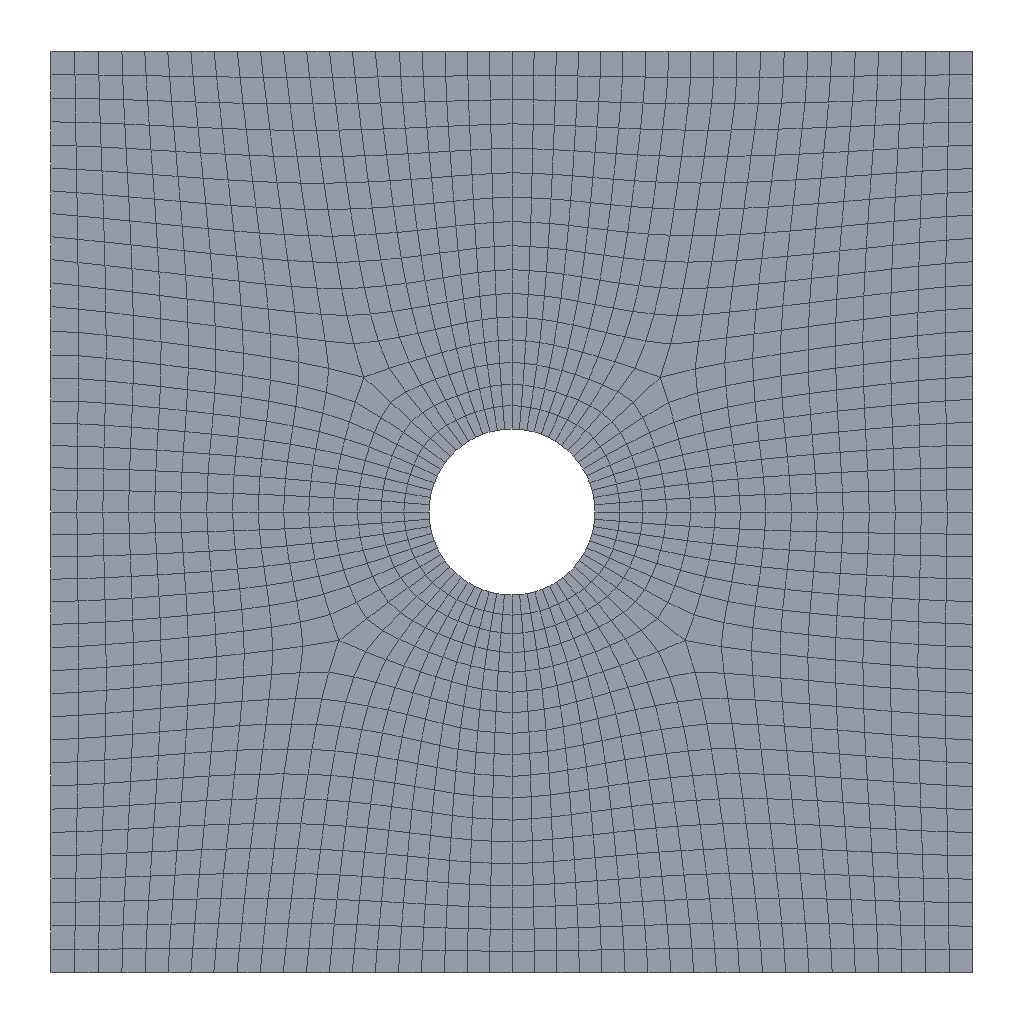Simulation study | abaqus
Set-up summary:
category,name,step,type,value,unit,region
solver,abaqus
solver,version,,,Abaqus/Standard 2020
units,not stated in the deck,,not stated
analysis,deck,,soils,soils
load_step,Step-1,Step-1,soils
load_step,requested,,,1
mesh,nodes,,,1736
mesh,elements,,,1622
element_type,CPE4P,,plane,1622
load,load commands in deck,,count,1
bc,support commands in deck,,count,2
material,MATERIAL-1,,in results
check,setup vs results,,match,"per instance, exact: element labels, types and connectivity; labels of the nodes the elements use; coordinates of those nodes at SINGLE_PRECISION in 1 of 1 instance(s)"
Abaqus input file, long lists of numbers shortened:
*Heading
** Job name: Job-1 Model name: Model-1
** Generated by: Abaqus/CAE 2020
*Preprint, echo=NO, model=NO, history=NO, contact=NO
**
** PARTS
**
*Part, name=Part-1
*Node
      1,        -400.,       -1200.
      2,        -400.,        -708.
** (1734 more lines like these left out)
*Element, type=CPE4P
  1,  88,  89, 330, 310
  2,  89,  90, 331, 330
** (1620 more lines like these left out)
*Nset, nset=Set-5, generate
    1,  1736,     1
*Elset, elset=Set-5, generate
    1,  1622,     1
** Section: Section-1
*Solid Section, elset=Set-5, material=Material-1
,
*End Part
**
**
** ASSEMBLY
**
*Assembly, name=Assembly
**
*Instance, name=Part-1-1, part=Part-1
*End Instance
**
*Nset, nset=Set-1, instance=Part-1-1
   4,   5,   6,   7,  11,  12,  60,  61,  62,  63,  64,  65,  66,  67,  68,  69
  70,  71,  72,  73,  74,  75,  76,  77,  78, 117, 118, 119, 120, 121, 122, 123
** (4 more lines like these left out)
*Elset, elset=Set-1, instance=Part-1-1
  225,  235,  245,  255,  265,  275,  285,  286,  287,  288,  289,  290,  291,  292,  293,  294
  295,  296,  297,  298,  605,  615,  625,  635,  645,  655,  665,  675,  685,  695,  705,  715
** (3 more lines like these left out)
*Nset, nset=Set-2, instance=Part-1-1
   1,   5,   6,  10,  11,  12,  79,  80,  81,  82,  83,  84,  85,  86,  87,  88
  89,  90,  91,  92,  93,  94,  95,  96,  97,  98,  99, 100, 101, 102, 103, 104
** (4 more lines like these left out)
*Elset, elset=Set-2, instance=Part-1-1
    1,    2,    3,    4,    5,    6,    7,    8,    9,   10,  298,  311,  324,  337,  350,  363
  376,  389,  402,  415,  478,  491,  504,  517,  530,  543,  556,  569,  582,  595,  596,  597
** (3 more lines like these left out)
*Nset, nset=Set-3, instance=Part-1-1, generate
    1,  1736,     1
*Elset, elset=Set-3, instance=Part-1-1, generate
    1,  1622,     1
*Nset, nset=Set-4, instance=Part-1-1
   2,   3,   8,   9,  30,  31,  32,  33,  34,  35,  36,  37,  38,  39,  40,  41
  42,  43,  44,  45, 150, 151, 152, 153, 154, 155, 156, 157, 158, 159, 160, 161
** (3 more lines like these left out)
*Elset, elset=Set-4, instance=Part-1-1
  135,  140,  145,  150,  155,  160,  165,  170,  175,  180,  181,  182,  183,  184,  185,  186
  187,  416,  417,  418,  419,  420,  421,  422,  423,  424,  425,  800,  805,  810,  815,  820
** (3 more lines like these left out)
*Nset, nset=Set-5, instance=Part-1-1, generate
    1,  1736,     1
*Elset, elset=Set-5, instance=Part-1-1, generate
    1,  1622,     1
*Nset, nset=Set-6, instance=Part-1-1
   1,   5,   6,  79,  80,  81,  82,  83,  84,  85,  86,  87,  88,  89,  90,  91
  92,  93,  94,  95,  96,  97,  98,  99, 100, 101, 102, 103, 104, 105, 106, 107
** (1 more lines like these left out)
*Elset, elset=Set-6, instance=Part-1-1
   1,   2,   3,   4,   5,   6,   7,   8,   9,  10, 298, 311, 324, 337, 350, 363
 376, 389, 402, 415, 478, 491, 504, 517, 530, 543, 556, 569, 582, 595, 596, 597
** (1 more lines like these left out)
*Nset, nset=Set-7, instance=Part-1-1
   1,   5,   6,  10,  11,  12,  79,  80,  81,  82,  83,  84,  85,  86,  87,  88
  89,  90,  91,  92,  93,  94,  95,  96,  97,  98,  99, 100, 101, 102, 103, 104
** (4 more lines like these left out)
*Elset, elset=Set-7, instance=Part-1-1
    1,    2,    3,    4,    5,    6,    7,    8,    9,   10,  298,  311,  324,  337,  350,  363
  376,  389,  402,  415,  478,  491,  504,  517,  530,  543,  556,  569,  582,  595,  596,  597
** (3 more lines like these left out)
*Nset, nset=Set-8, instance=Part-1-1
  10,  11,  12, 181, 182, 183, 184, 185, 186, 187, 188, 189, 190, 191, 192, 193
 194, 195, 196, 197, 198, 199, 270, 271, 272, 273, 274, 275, 276, 277, 278, 279
** (1 more lines like these left out)
*Elset, elset=Set-8, instance=Part-1-1
  878,  890,  902,  914,  926,  938,  950,  962,  974,  975,  976,  977,  978,  979,  980,  981
  982,  983,  984,  985, 1227, 1228, 1229, 1230, 1231, 1232, 1233, 1234, 1235, 1502, 1514, 1526
** (1 more lines like these left out)
*Nset, nset=Set-9, instance=Part-1-1, generate
    1,  1736,     1
*Elset, elset=Set-9, instance=Part-1-1, generate
    1,  1622,     1
*Nset, nset=Set-10, instance=Part-1-1
   1,   5,   6,  10,  11,  12,  79,  80,  81,  82,  83,  84,  85,  86,  87,  88
  89,  90,  91,  92,  93,  94,  95,  96,  97,  98,  99, 100, 101, 102, 103, 104
** (4 more lines like these left out)
*Elset, elset=Set-10, instance=Part-1-1
    1,    2,    3,    4,    5,    6,    7,    8,    9,   10,  298,  311,  324,  337,  350,  363
  376,  389,  402,  415,  478,  491,  504,  517,  530,  543,  556,  569,  582,  595,  596,  597
** (3 more lines like these left out)
*Elset, elset=_Surf-1_S2, internal, instance=Part-1-1
  135,  140,  145,  150,  155,  160,  165,  170,  175,  180,  800,  805,  810,  815,  820,  825
  830, 1198, 1202, 1206, 1210, 1214, 1218, 1222, 1226, 1338, 1342, 1346, 1350, 1354, 1358, 1362
** (1 more lines like these left out)
*Elset, elset=_Surf-1_S1, internal, instance=Part-1-1
  181,  182,  183,  184,  185,  186,  187,  416,  417,  418,  419,  420,  421,  422,  423,  424
  425,  831,  832,  833,  834,  835,  836,  837,  838,  839, 1371, 1372, 1373, 1374, 1375, 1376
** (1 more lines like these left out)
*Surface, type=ELEMENT, name=Surf-1
_Surf-1_S2, S2
_Surf-1_S1, S1
*Elset, elset=_Surf-2_S2, internal, instance=Part-1-1
  135,  140,  145,  150,  155,  160,  165,  170,  175,  180,  800,  805,  810,  815,  820,  825
  830, 1198, 1202, 1206, 1210, 1214, 1218, 1222, 1226, 1338, 1342, 1346, 1350, 1354, 1358, 1362
** (1 more lines like these left out)
*Elset, elset=_Surf-2_S1, internal, instance=Part-1-1
  181,  182,  183,  184,  185,  186,  187,  416,  417,  418,  419,  420,  421,  422,  423,  424
  425,  831,  832,  833,  834,  835,  836,  837,  838,  839, 1371, 1372, 1373, 1374, 1375, 1376
** (1 more lines like these left out)
*Surface, type=ELEMENT, name=Surf-2
_Surf-2_S2, S2
_Surf-2_S1, S1
*Elset, elset=_Surf-3_S2, internal, instance=Part-1-1
  878,  890,  902,  914,  926,  938,  950,  962,  974, 1502, 1514, 1526, 1538, 1550, 1562, 1574
 1586, 1598, 1610, 1622
*Elset, elset=_Surf-3_S1, internal, instance=Part-1-1
  975,  976,  977,  978,  979,  980,  981,  982,  983,  984,  985, 1227, 1228, 1229, 1230, 1231
 1232, 1233, 1234, 1235
*Surface, type=ELEMENT, name=Surf-3
_Surf-3_S2, S2
_Surf-3_S1, S1
*Elset, elset=_Surf-4_S1, internal, instance=Part-1-1
    1,    2,    3,    4,    5,    6,    7,    8,    9,   10,  596,  597,  598,  599,  600,  601
  602,  603,  604,  605,  975,  976,  977,  978,  979,  980,  981,  982,  983,  984,  985, 1227
** (1 more lines like these left out)
*Elset, elset=_Surf-4_S2, internal, instance=Part-1-1
  298,  311,  324,  337,  350,  363,  376,  389,  402,  415,  478,  491,  504,  517,  530,  543
  556,  569,  582,  595,  878,  890,  902,  914,  926,  938,  950,  962,  974, 1502, 1514, 1526
** (1 more lines like these left out)
*Surface, type=ELEMENT, name=Surf-4
_Surf-4_S1, S1
_Surf-4_S2, S2
*Elset, elset=_Surf-5_S2, internal, instance=Part-1-1
  225,  235,  245,  255,  265,  275,  285,  605,  615,  625,  635,  645,  655,  665,  675,  685
  695,  705,  715,  725,  985,  996, 1007, 1018, 1029, 1040, 1051, 1062, 1073, 1084, 1095, 1106
** (1 more lines like these left out)
*Elset, elset=_Surf-5_S1, internal, instance=Part-1-1
  286,  287,  288,  289,  290,  291,  292,  293,  294,  295,  296,  297,  298,  726,  727,  728
  729,  730,  731,  732, 1107, 1108, 1109, 1110, 1111, 1112, 1113, 1114, 1491, 1492, 1493, 1494
** (1 more lines like these left out)
*Surface, type=ELEMENT, name=Surf-5
_Surf-5_S2, S2
_Surf-5_S1, S1
*End Assembly
*Amplitude, name=Amp-1
             0.,              0.,              1.,              1.
**
** MATERIALS
**
*Material, name=Material-1
*Elastic
 2e+10, 0.2
*Fluid Leakoff
 1e-14, 1e-14
*Gap Flow
 0.001,
*Permeability, specific=9800.
 1e-08, 0.2
*Mohr Coulomb
20., 0.1
*Mohr Coulomb Hardening
 1e+07,0.
**
** PREDEFINED FIELDS
**
** Name: Predefined Field-1   Type: Void ratio
*Initial Conditions, TYPE=RATIO
Set-3, 0.03
** Name: Predefined Field-2   Type: Stress
*Initial Conditions, type=STRESS
Set-5, 1e+06, 1.11e+07, 0., 0.,
** ----------------------------------------------------------------
**
** STEP: Step-1
**
*Step, name=Step-1, nlgeom=YES, inc=1000
*Soils, utol=1.0, stabilize=0.0002, allsdtol=0.05, continue=NO
0.001, 100., 0.001, 100.,
**
** BOUNDARY CONDITIONS
**
** Name: BC-1 Type: 位移/转角
*Boundary
Set-1, 1, 1
** Name: BC-2 Type: 位移/转角
*Boundary
Set-7, 2, 2
**
** LOADS
**
** Name: Load-1   Type: Pressure
*Dsload
Surf-2, P, 1.4e+07
**
** OUTPUT REQUESTS
**
*Restart, write, frequency=0
**
** FIELD OUTPUT: F-Output-1
**
*Output, field
*Node Output
CF, POR, RF, U, V
*Element Output, directions=YES
E, EE, FLUVR, FLVEL, IE, LE, MISES, PE, PEEQ, PEEQMAX, PEEQT, PEMAG, PEQC, S, SAT, VE
VEEQ, VOIDR
*Contact Output
PFL, PFLA, PTL, PTLA
**
** HISTORY OUTPUT: H-Output-1
**
*Output, history, variable=PRESELECT
*End Step
Results summary:
result,step,,completed,increments=30 time=100.0/100.0
result,analysis,,,soils
result,last_loadstep,,,1
result,primary field,,,"U, POR"
result,reaction total,,FX,-14.75,model units
result,reaction total,,FY,0.0,model units
result,reaction total,,FZ,0.0,model units